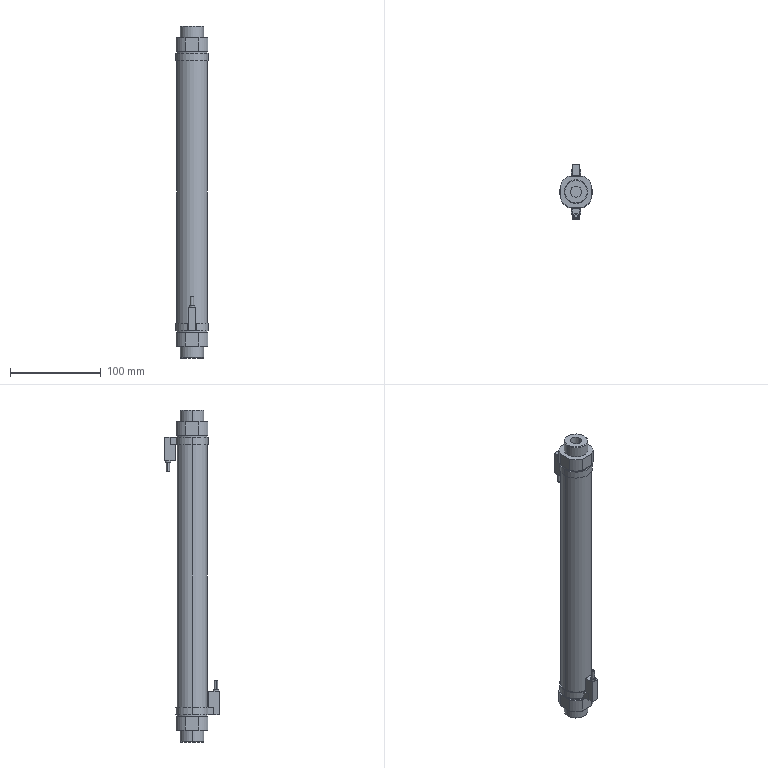Part | STEP file | body_A_CDM2B32_275_C76_0_ | 1 solid | 96 faces | box 35.8 x 59.8 x 365 mm | volume 294811 mm3 | plane 48 | cylinder 40 | cone 8 | commonest cylinder face diameters 35.8 x8 37.5 x8 33.8 x6 3.4 x4 6 x4 8.57 x4